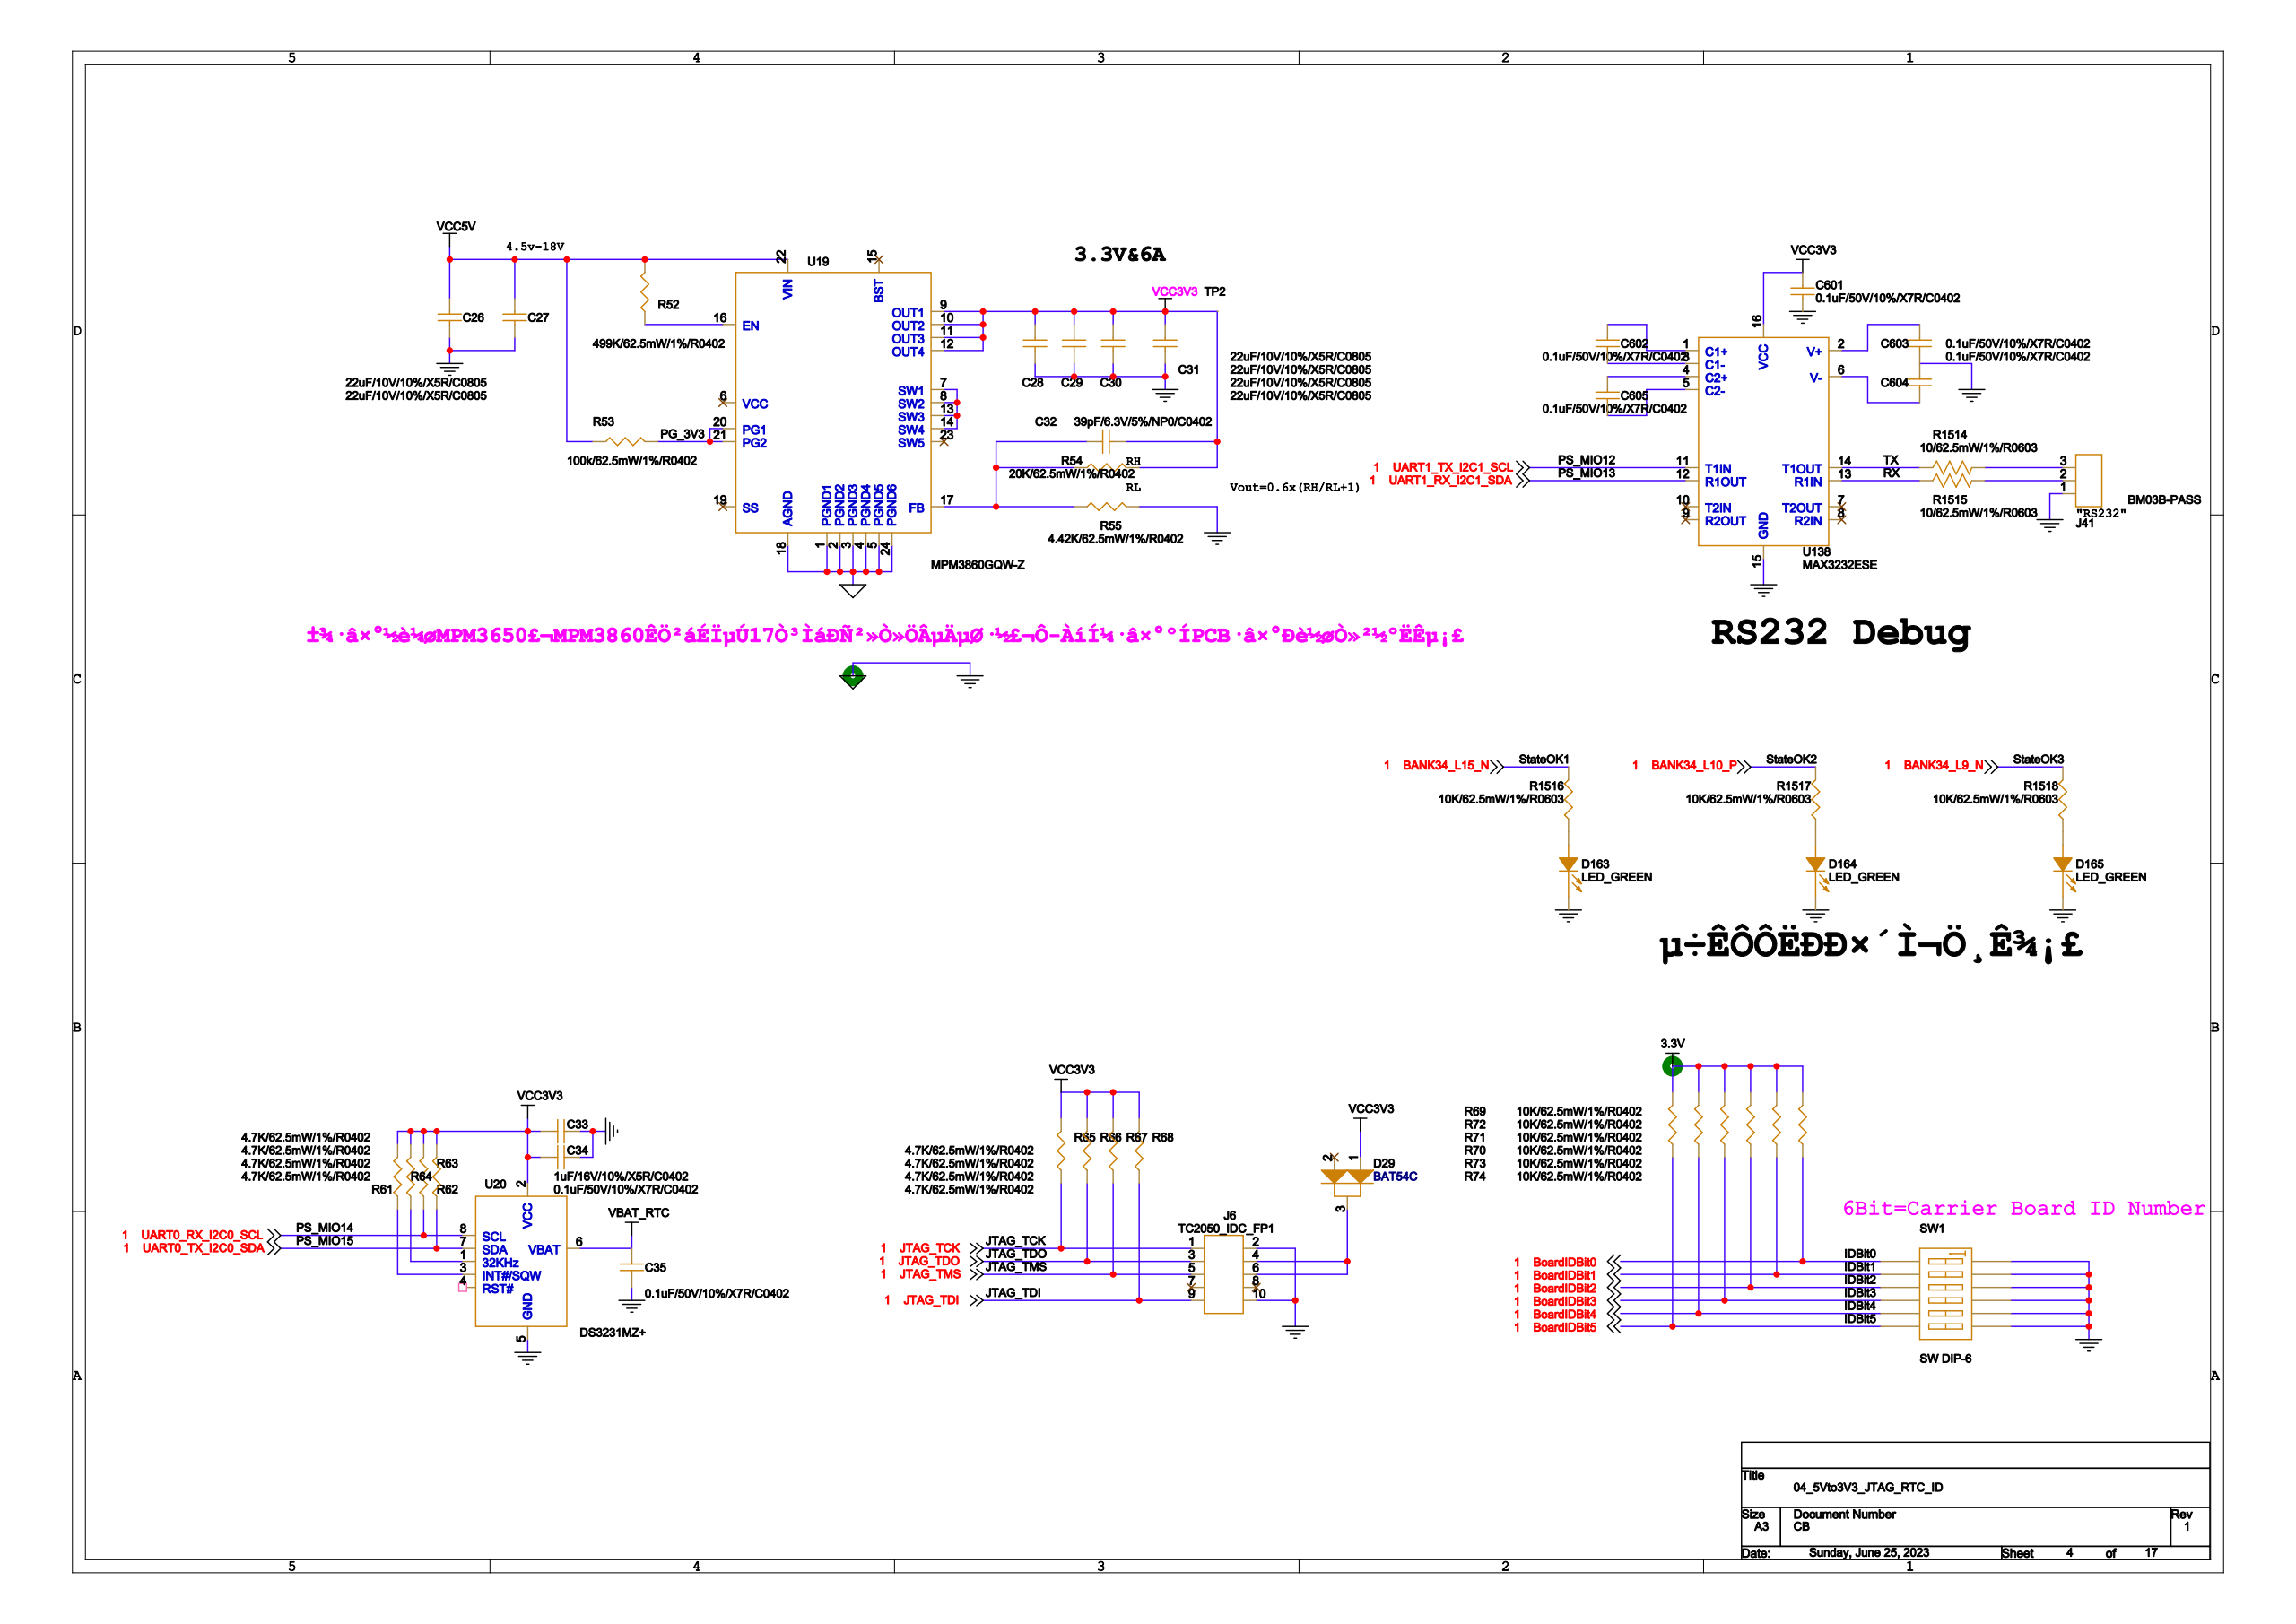Circuit board | Cadence Allegro | 1997 parts | 1536 nets | one sheet of the schematic
Parts on this sheet (reference | value | footprint):
C26 | 22uF/10V/10%/X5R/C0805 | 0805
C27 | 22uF/10V/10%/X5R/C0805 | 0805
C28 | 22uF/10V/10%/X5R/C0805 | 0805
C29 | 22uF/10V/10%/X5R/C0805 | 0805
C30 | 22uF/10V/10%/X5R/C0805 | 0805
C31 | 22uF/10V/10%/X5R/C0805 | 0805
C32 | 39pF/6.3V/5%/NP0/C0402 | 0402
C33 | 1uF/16V/10%/X5R/C0402 | 0402
C34 | 0.1uF/50V/10%/X7R/C0402 | 0402
C35 | 0.1uF/50V/10%/X7R/C0402 | 0402
C601 | 0.1uF/50V/10%/X7R/C0402 | 0402
C602 | 0.1uF/50V/10%/X7R/C0402 | 0402
C603 | 0.1uF/50V/10%/X7R/C0402 | 0402
C604 | 0.1uF/50V/10%/X7R/C0402 | 0402
C605 | 0.1uF/50V/10%/X7R/C0402 | 0402
D29 | BAT54C | SOT23
D163 | LED_GREEN | LED0805
D164 | LED_GREEN | LED0805
D165 | LED_GREEN | LED0805
J6 | TC2050_IDC_FP1 | IDC-TH_Z-231012810106
J41 | BM03B-PASS | BM03B-PASS
R52 | 499K/62.5mW/1%/R0402 | 0402
R53 | 100k/62.5mW/1%/R0402 | 0402
R54 | 20K/62.5mW/1%/R0402 | 0402
R55 | 4.42K/62.5mW/1%/R0402 | 0402
R61 | 4.7K/62.5mW/1%/R0402 | 0402
R62 | 4.7K/62.5mW/1%/R0402 | 0402
R63 | 4.7K/62.5mW/1%/R0402 | 0402
R64 | 4.7K/62.5mW/1%/R0402 | 0402
R65 | 4.7K/62.5mW/1%/R0402 | 0402
R66 | 4.7K/62.5mW/1%/R0402 | 0402
R67 | 4.7K/62.5mW/1%/R0402 | 0402
R68 | 4.7K/62.5mW/1%/R0402 | 0402
R69 | 10K/62.5mW/1%/R0402 | 0402
R70 | 10K/62.5mW/1%/R0402 | 0402
R71 | 10K/62.5mW/1%/R0402 | 0402
R72 | 10K/62.5mW/1%/R0402 | 0402
R73 | 10K/62.5mW/1%/R0402 | 0402
R74 | 10K/62.5mW/1%/R0402 | 0402
R1514 | 10/62.5mW/1%/R0603 | 0603R
R1515 | 10/62.5mW/1%/R0603 | 0603R
R1516 | 10K/62.5mW/1%/R0603 | 0603R
R1517 | 10K/62.5mW/1%/R0603 | 0603R
R1518 | 10K/62.5mW/1%/R0603 | 0603R
SW1 | SW DIP-6 | W-SMD_12P-L9_3-W5_4-P1_27-LS2
TP2 | TEST POINT A | TEST_12MM
U19 | MPM3860GQW-Z | MPM3650GQW
U20 | DS3231MZ+ | SO8
U138 | MAX3232ESE | SO16
Nets of these parts (net: part-pin ...):
3.3V: C28-1 C29-1 C30-1 C31-1 C32-2 C33-2 C34-2 C601-1 D29-1 R54-1 R61-1 R62-1 R63-1 R64-1 R65-1 R66-1 R67-1 R68-1 R69-1 R70-1 R71-1 R72-1 R73-1 R74-1 TP2-1 U19-9 U19-10 U19-11 U19-12 U20-2 U138-16
AGND: C26-2 C27-2 C28-2 C29-2 C30-2 C31-2 C33-1 C34-1 C35-2 C601-2 C603-2 C604-1 D163-2 D164-2 D165-2 J6-2 J6-10 J41-1 R55-1 SW1-7 SW1-8 SW1-9 SW1-10 SW1-11 SW1-12 U19-1 U19-2 U19-3 U19-4 U19-5 U19-18 U19-24 U20-5 U138-15
BOARDIDBIT0: R74-2 SW1-1
BOARDIDBIT1: R73-2 SW1-2
BOARDIDBIT2: R72-2 SW1-3
BOARDIDBIT3: R71-2 SW1-4
BOARDIDBIT4: R70-2 SW1-5
BOARDIDBIT5: R69-2 SW1-6
BANK34_L9_N: R1518-2
BANK34_L10_P: R1517-2
VCC5V: C26-1 C27-1 R52-1 R53-2 U19-22
BANK34_L15_N: R1516-2
JTAG_TDO: J6-3 R66-2
JTAG_TMS: J6-5 R67-2
JTAG_TDI: J6-9 R68-2
JTAG_TCK: J6-1 R65-2
UART0_RX_I2C0_SCL: R63-2 U20-8
UART0_TX_I2C0_SDA: R64-2 U20-7
UART1_TX_I2C1_SCL: U138-11
UART1_RX_I2C1_SDA: U138-12
N23857910: D29-3 J6-4 J6-6
N23931017: J41-2 R1515-2
N23931015: J41-3 R1514-2
N23930865: C602-1 U138-1
N23930898: C602-2 U138-3
N23930926: C605-1 U138-4
N23930940: C605-2 U138-5
RX: R1515-1 U138-13
TX: R1514-1 U138-14
N23930874: C603-1 U138-2
N23930928: C604-2 U138-6
N239315640: D163-1 R1516-1
N239315840: D164-1 R1517-1
N239316020: D165-1 R1518-1
VBAT_RTC: C35-1 U20-6
N23155169: C32-1 R54-2 R55-2 U19-17
N23155064: R52-2 U19-16
PG_3V3: R53-1 U19-20 U19-21
N23857516: R61-2 U20-3
N23857518: R62-2 U20-1
N23155134: U19-7 U19-8 U19-13 U19-14